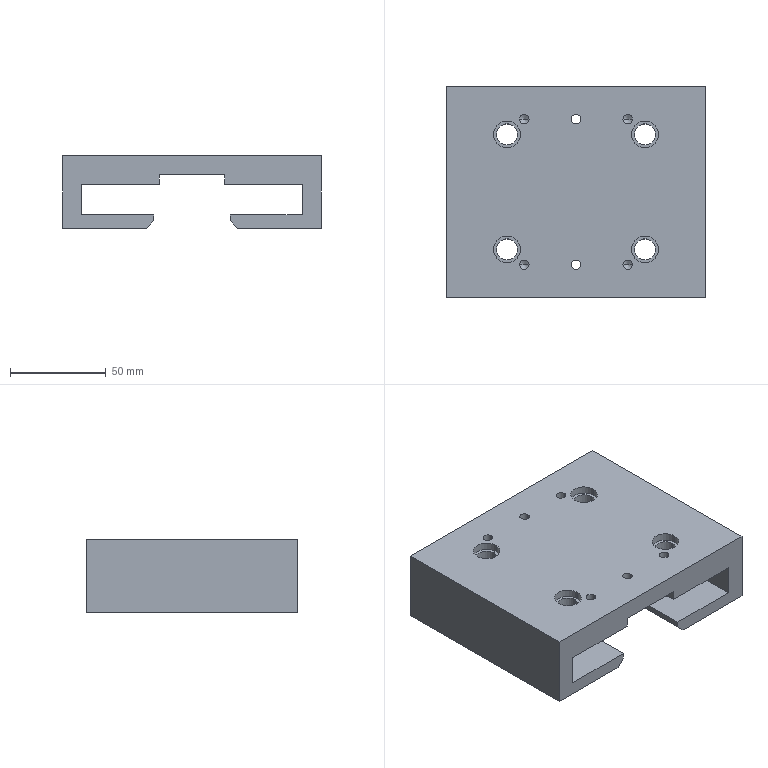Part | SolidWorks | features ICE 4, LPattern 2, Chamfer 1, Extrusion 1, HoleWzd 1 | 1 solid | 80 faces | box 135 x 110 x 38 mm | volume 295400 mm3 | cylinder 44 | plane 28 | cone 8 | commonest cylinder face diameters 11 x16 5 x12 14 x8 22 x8